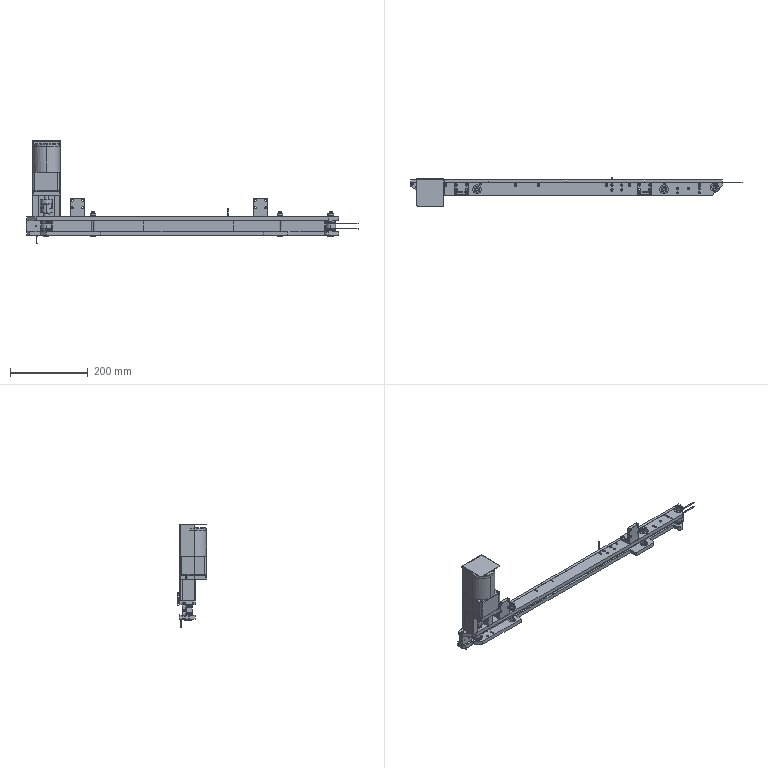Part | NX | 59 solids | 2005 faces | box 852 x 75.7 x 266.393 mm | volume 1375290 mm3 | cylinder 902 | cone 520 | plane 507 | torus 62 | spline 14 | commonest cylinder face diameters 2.5 x134 3.3 x130 4.2 x70 3.5 x60 6 x58 5.5 x56